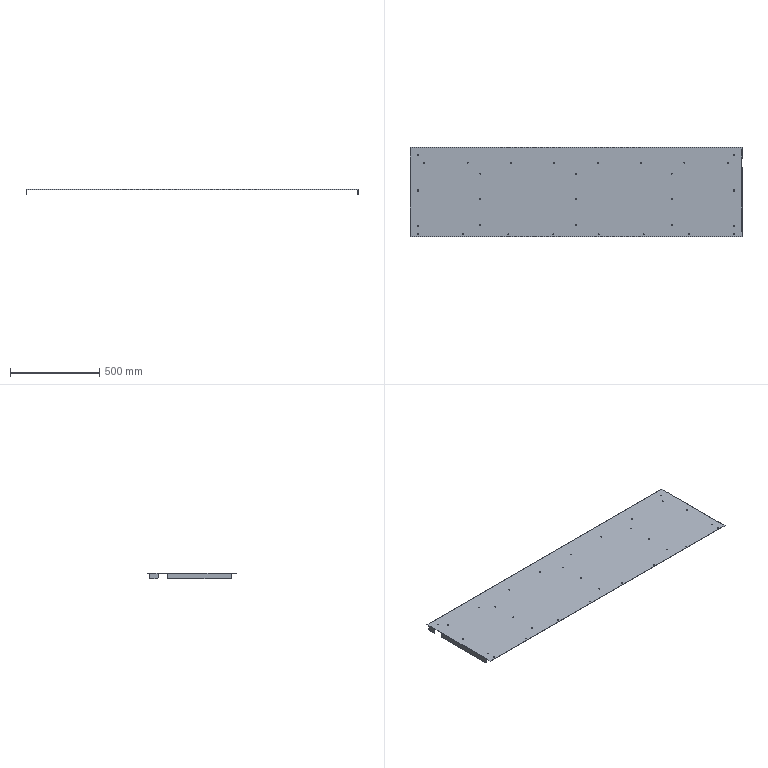Part | STEP file | SX-S26 | 1 solid | 118 faces | box 1865 x 502.5 x 30 mm | volume 1150989 mm3 | cylinder 78 | plane 40 | commonest cylinder face diameters 5.4 x54 6.4 x8 10 x8 0.4 x4 2.8 x4